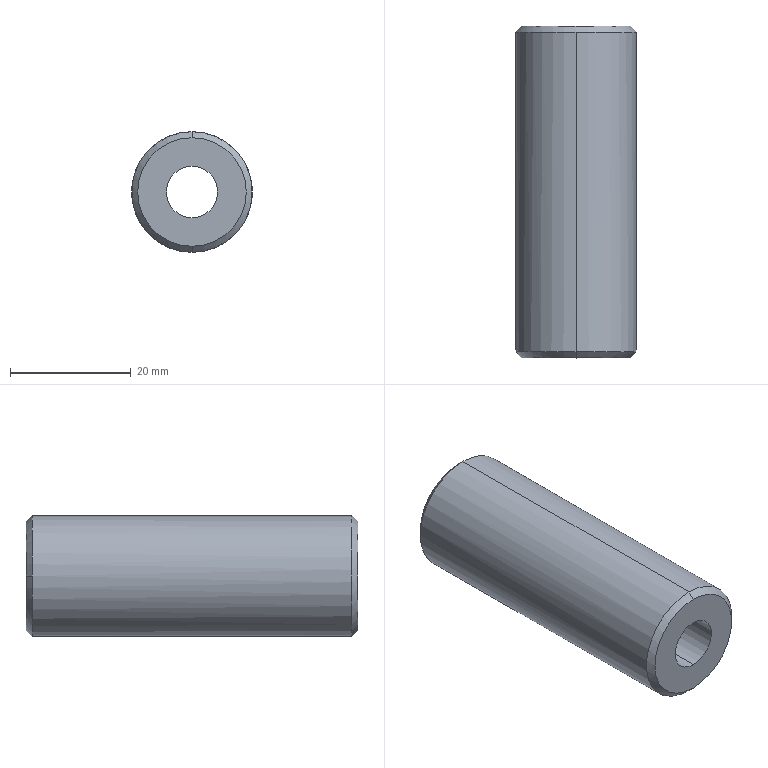Part | SolidWorks | features BaseBody 1 | 1 solid | 10 faces | box 20 x 55 x 20 mm | volume 14097 mm3 | cylinder 4 | cone 4 | plane 2 | commonest cylinder face diameters 8.5 x2 20 x2
STEP:
#1=CARTESIAN_POINT('',(10.,54.,0.));
#2=VERTEX_POINT('',#1);
#3=CARTESIAN_POINT('',(0.,54.,10.));
#4=VERTEX_POINT('',#3);
#5=CARTESIAN_POINT('',(0.,54.,0.));
#6=DIRECTION('',(0.,-1.,0.));
#7=DIRECTION('',(0.,0.,-1.));
#8=AXIS2_PLACEMENT_3D('',#5,#6,#7);
#9=CIRCLE('',#8,10.);
#10=EDGE_CURVE('',#2,#4,#9,.T.);
#11=ORIENTED_EDGE('',*,*,#10,.T.);
#12=CARTESIAN_POINT('',(0.,1.,10.));
#13=VERTEX_POINT('',#12);
#14=CARTESIAN_POINT('',(0.,55.,10.));
#15=DIRECTION('',(0.,-1.,0.));
#16=VECTOR('',#15,1000.);
#17=LINE('',#14,#16);
#18=EDGE_CURVE('',#4,#13,#17,.T.);
#19=ORIENTED_EDGE('',*,*,#18,.T.);
#20=CARTESIAN_POINT('',(0.,1.,-10.));
#21=VERTEX_POINT('',#20);
#22=CARTESIAN_POINT('',(0.,1.,0.));
#23=DIRECTION('',(0.,1.,0.));
#24=DIRECTION('',(0.,0.,-1.));
#25=AXIS2_PLACEMENT_3D('',#22,#23,#24);
#26=CIRCLE('',#25,10.);
#27=EDGE_CURVE('',#13,#21,#26,.T.);
#28=ORIENTED_EDGE('',*,*,#27,.T.);
#29=CARTESIAN_POINT('',(0.,54.,-10.));
#30=VERTEX_POINT('',#29);
#31=CARTESIAN_POINT('',(0.,55.,-10.));
#32=DIRECTION('',(0.,-1.,0.));
#33=VECTOR('',#32,1000.);
#34=LINE('',#31,#33);
#35=EDGE_CURVE('',#30,#21,#34,.T.);
#36=ORIENTED_EDGE('',*,*,#35,.F.);
#37=CARTESIAN_POINT('',(0.,54.,0.));
#38=DIRECTION('',(0.,-1.,0.));
#39=DIRECTION('',(0.,0.,-1.));
#40=AXIS2_PLACEMENT_3D('',#37,#38,#39);
#41=CIRCLE('',#40,10.);
#42=EDGE_CURVE('',#30,#2,#41,.T.);
#43=ORIENTED_EDGE('',*,*,#42,.T.);
#44=EDGE_LOOP('',(#11,#19,#28,#36,#43));
#45=FACE_OUTER_BOUND('',#44,.T.);
#46=CARTESIAN_POINT('',(0.,55.,0.));
#47=DIRECTION('',(0.,-1.,0.));
#48=DIRECTION('',(0.,0.,-1.));
#49=AXIS2_PLACEMENT_3D('',#46,#47,#48);
#50=CYLINDRICAL_SURFACE('',#49,10.);
#51=ADVANCED_FACE('',(#45),#50,.T.);
#52=CARTESIAN_POINT('',(0.,0.,9.));
#53=VERTEX_POINT('',#52);
#54=CARTESIAN_POINT('',(0.,0.,-9.));
#55=VERTEX_POINT('',#54);
#56=CARTESIAN_POINT('',(0.,0.,0.));
#57=DIRECTION('',(0.,1.,0.));
#58=DIRECTION('',(0.,0.,1.));
#59=AXIS2_PLACEMENT_3D('',#56,#57,#58);
#60=CIRCLE('',#59,9.);
#61=EDGE_CURVE('',#53,#55,#60,.T.);
#62=ORIENTED_EDGE('',*,*,#61,.T.);
#63=CARTESIAN_POINT('',(0.,1.,-10.));
#64=DIRECTION('',(0.,0.7071,-0.7071));
#65=VECTOR('',#64,1000.);
#66=LINE('',#63,#65);
#67=EDGE_CURVE('',#55,#21,#66,.T.);
#68=ORIENTED_EDGE('',*,*,#67,.T.);
#69=ORIENTED_EDGE('',*,*,#27,.F.);
#70=CARTESIAN_POINT('',(0.,1.,10.));
#71=DIRECTION('',(0.,0.7071,0.7071));
#72=VECTOR('',#71,1000.);
#73=LINE('',#70,#72);
#74=EDGE_CURVE('',#53,#13,#73,.T.);
#75=ORIENTED_EDGE('',*,*,#74,.F.);
#76=EDGE_LOOP('',(#62,#68,#69,#75));
#77=FACE_OUTER_BOUND('',#76,.T.);
#78=CARTESIAN_POINT('',(0.,1.,0.));
#79=DIRECTION('',(0.,1.,0.));
#80=DIRECTION('',(0.,0.,1.));
#81=AXIS2_PLACEMENT_3D('',#78,#79,#80);
#82=CONICAL_SURFACE('',#81,10.,0.7854);
#83=ADVANCED_FACE('',(#77),#82,.T.);
#84=CARTESIAN_POINT('',(9.,55.,0.));
#85=VERTEX_POINT('',#84);
#86=CARTESIAN_POINT('',(-9.,55.,0.));
#87=VERTEX_POINT('',#86);
#88=CARTESIAN_POINT('',(0.,55.,0.));
#89=DIRECTION('',(0.,-1.,0.));
#90=DIRECTION('',(1.,0.,0.));
#91=AXIS2_PLACEMENT_3D('',#88,#89,#90);
#92=CIRCLE('',#91,9.);
#93=EDGE_CURVE('',#85,#87,#92,.T.);
#94=ORIENTED_EDGE('',*,*,#93,.T.);
#95=CARTESIAN_POINT('',(-10.,54.,0.));
#96=VERTEX_POINT('',#95);
#97=CARTESIAN_POINT('',(-10.,54.,0.));
#98=DIRECTION('',(-0.7071,-0.7071,0.));
#99=VECTOR('',#98,1000.);
#100=LINE('',#97,#99);
#101=EDGE_CURVE('',#87,#96,#100,.T.);
#102=ORIENTED_EDGE('',*,*,#101,.T.);
#103=CARTESIAN_POINT('',(0.,54.,0.));
#104=DIRECTION('',(0.,-1.,0.));
#105=DIRECTION('',(0.,0.,-1.));
#106=AXIS2_PLACEMENT_3D('',#103,#104,#105);
#107=CIRCLE('',#106,10.);
#108=EDGE_CURVE('',#4,#96,#107,.T.);
#109=ORIENTED_EDGE('',*,*,#108,.F.);
#110=ORIENTED_EDGE('',*,*,#10,.F.);
#111=CARTESIAN_POINT('',(10.,54.,0.));
#112=DIRECTION('',(0.7071,-0.7071,0.));
#113=VECTOR('',#112,1000.);
#114=LINE('',#111,#113);
#115=EDGE_CURVE('',#85,#2,#114,.T.);
#116=ORIENTED_EDGE('',*,*,#115,.F.);
#117=EDGE_LOOP('',(#94,#102,#109,#110,#116));
#118=FACE_OUTER_BOUND('',#117,.T.);
#119=CARTESIAN_POINT('',(0.,54.,0.));
#120=DIRECTION('',(0.,-1.,0.));
#121=DIRECTION('',(1.,0.,0.));
#122=AXIS2_PLACEMENT_3D('',#119,#120,#121);
#123=CONICAL_SURFACE('',#122,10.,0.7854);
#124=ADVANCED_FACE('',(#118),#123,.T.);
#125=CARTESIAN_POINT('',(0.,0.,4.25));
#126=VERTEX_POINT('',#125);
#127=CARTESIAN_POINT('',(0.,0.,-4.25));
#128=VERTEX_POINT('',#127);
#129=CARTESIAN_POINT('',(0.,0.,0.));
#130=DIRECTION('',(0.,-1.,0.));
#131=DIRECTION('',(0.,0.,1.));
#132=AXIS2_PLACEMENT_3D('',#129,#130,#131);
#133=CIRCLE('',#132,4.25);
#134=EDGE_CURVE('',#126,#128,#133,.T.);
#135=ORIENTED_EDGE('',*,*,#134,.T.);
#136=CARTESIAN_POINT('',(0.,55.,-4.25));
#137=VERTEX_POINT('',#136);
#138=CARTESIAN_POINT('',(0.,55.,-4.25));
#139=DIRECTION('',(0.,1.,0.));
#140=VECTOR('',#139,1000.);
#141=LINE('',#138,#140);
#142=EDGE_CURVE('',#128,#137,#141,.T.);
#143=ORIENTED_EDGE('',*,*,#142,.T.);
#144=CARTESIAN_POINT('',(0.,55.,4.25));
#145=VERTEX_POINT('',#144);
#146=CARTESIAN_POINT('',(0.,55.,0.));
#147=DIRECTION('',(0.,-1.,0.));
#148=DIRECTION('',(0.,0.,1.));
#149=AXIS2_PLACEMENT_3D('',#146,#147,#148);
#150=CIRCLE('',#149,4.25);
#151=EDGE_CURVE('',#145,#137,#150,.T.);
#152=ORIENTED_EDGE('',*,*,#151,.F.);
#153=CARTESIAN_POINT('',(0.,55.,4.25));
#154=DIRECTION('',(0.,1.,0.));
#155=VECTOR('',#154,1000.);
#156=LINE('',#153,#155);
#157=EDGE_CURVE('',#126,#145,#156,.T.);
#158=ORIENTED_EDGE('',*,*,#157,.F.);
#159=EDGE_LOOP('',(#135,#143,#152,#158));
#160=FACE_OUTER_BOUND('',#159,.T.);
#161=CARTESIAN_POINT('',(0.,55.,0.));
#162=DIRECTION('',(0.,1.,0.));
#163=DIRECTION('',(0.,0.,1.));
#164=AXIS2_PLACEMENT_3D('',#161,#162,#163);
#165=CYLINDRICAL_SURFACE('',#164,4.25);
#166=ADVANCED_FACE('',(#160),#165,.F.);
#167=ORIENTED_EDGE('',*,*,#18,.F.);
#168=ORIENTED_EDGE('',*,*,#108,.T.);
#169=CARTESIAN_POINT('',(0.,54.,0.));
#170=DIRECTION('',(0.,-1.,0.));
#171=DIRECTION('',(0.,0.,-1.));
#172=AXIS2_PLACEMENT_3D('',#169,#170,#171);
#173=CIRCLE('',#172,10.);
#174=EDGE_CURVE('',#96,#30,#173,.T.);
#175=ORIENTED_EDGE('',*,*,#174,.T.);
#176=ORIENTED_EDGE('',*,*,#35,.T.);
#177=CARTESIAN_POINT('',(0.,1.,0.));
#178=DIRECTION('',(0.,1.,0.));
#179=DIRECTION('',(0.,0.,-1.));
#180=AXIS2_PLACEMENT_3D('',#177,#178,#179);
#181=CIRCLE('',#180,10.);
#182=EDGE_CURVE('',#21,#13,#181,.T.);
#183=ORIENTED_EDGE('',*,*,#182,.T.);
#184=EDGE_LOOP('',(#167,#168,#175,#176,#183));
#185=FACE_OUTER_BOUND('',#184,.T.);
#186=CARTESIAN_POINT('',(0.,55.,0.));
#187=DIRECTION('',(0.,-1.,0.));
#188=DIRECTION('',(0.,0.,-1.));
#189=AXIS2_PLACEMENT_3D('',#186,#187,#188);
#190=CYLINDRICAL_SURFACE('',#189,10.);
#191=ADVANCED_FACE('',(#185),#190,.T.);
#192=ORIENTED_EDGE('',*,*,#67,.F.);
#193=CARTESIAN_POINT('',(0.,0.,0.));
#194=DIRECTION('',(0.,1.,0.));
#195=DIRECTION('',(0.,0.,1.));
#196=AXIS2_PLACEMENT_3D('',#193,#194,#195);
#197=CIRCLE('',#196,9.);
#198=EDGE_CURVE('',#55,#53,#197,.T.);
#199=ORIENTED_EDGE('',*,*,#198,.T.);
#200=ORIENTED_EDGE('',*,*,#74,.T.);
#201=ORIENTED_EDGE('',*,*,#182,.F.);
#202=EDGE_LOOP('',(#192,#199,#200,#201));
#203=FACE_OUTER_BOUND('',#202,.T.);
#204=CARTESIAN_POINT('',(0.,1.,0.));
#205=DIRECTION('',(0.,1.,0.));
#206=DIRECTION('',(0.,0.,1.));
#207=AXIS2_PLACEMENT_3D('',#204,#205,#206);
#208=CONICAL_SURFACE('',#207,10.,0.7854);
#209=ADVANCED_FACE('',(#203),#208,.T.);
#210=ORIENTED_EDGE('',*,*,#101,.F.);
#211=CARTESIAN_POINT('',(0.,55.,0.));
#212=DIRECTION('',(0.,-1.,0.));
#213=DIRECTION('',(1.,0.,0.));
#214=AXIS2_PLACEMENT_3D('',#211,#212,#213);
#215=CIRCLE('',#214,9.);
#216=EDGE_CURVE('',#87,#85,#215,.T.);
#217=ORIENTED_EDGE('',*,*,#216,.T.);
#218=ORIENTED_EDGE('',*,*,#115,.T.);
#219=ORIENTED_EDGE('',*,*,#42,.F.);
#220=ORIENTED_EDGE('',*,*,#174,.F.);
#221=EDGE_LOOP('',(#210,#217,#218,#219,#220));
#222=FACE_OUTER_BOUND('',#221,.T.);
#223=CARTESIAN_POINT('',(0.,54.,0.));
#224=DIRECTION('',(0.,-1.,0.));
#225=DIRECTION('',(1.,0.,0.));
#226=AXIS2_PLACEMENT_3D('',#223,#224,#225);
#227=CONICAL_SURFACE('',#226,10.,0.7854);
#228=ADVANCED_FACE('',(#222),#227,.T.);
#229=ORIENTED_EDGE('',*,*,#134,.F.);
#230=CARTESIAN_POINT('',(0.,0.,0.));
#231=DIRECTION('',(0.,-1.,0.));
#232=DIRECTION('',(0.,0.,1.));
#233=AXIS2_PLACEMENT_3D('',#230,#231,#232);
#234=CIRCLE('',#233,4.25);
#235=EDGE_CURVE('',#128,#126,#234,.T.);
#236=ORIENTED_EDGE('',*,*,#235,.F.);
#237=EDGE_LOOP('',(#229,#236));
#238=FACE_BOUND('',#237,.T.);
#239=ORIENTED_EDGE('',*,*,#61,.F.);
#240=ORIENTED_EDGE('',*,*,#198,.F.);
#241=EDGE_LOOP('',(#239,#240));
#242=FACE_OUTER_BOUND('',#241,.T.);
#243=CARTESIAN_POINT('',(0.,0.,0.));
#244=DIRECTION('',(0.,1.,0.));
#245=DIRECTION('',(0.,0.,1.));
#246=AXIS2_PLACEMENT_3D('',#243,#244,#245);
#247=PLANE('',#246);
#248=ADVANCED_FACE('',(#238,#242),#247,.F.);
#249=ORIENTED_EDGE('',*,*,#151,.T.);
#250=CARTESIAN_POINT('',(0.,55.,0.));
#251=DIRECTION('',(0.,-1.,0.));
#252=DIRECTION('',(0.,0.,1.));
#253=AXIS2_PLACEMENT_3D('',#250,#251,#252);
#254=CIRCLE('',#253,4.25);
#255=EDGE_CURVE('',#137,#145,#254,.T.);
#256=ORIENTED_EDGE('',*,*,#255,.T.);
#257=EDGE_LOOP('',(#249,#256));
#258=FACE_BOUND('',#257,.T.);
#259=ORIENTED_EDGE('',*,*,#93,.F.);
#260=ORIENTED_EDGE('',*,*,#216,.F.);
#261=EDGE_LOOP('',(#259,#260));
#262=FACE_OUTER_BOUND('',#261,.T.);
#263=CARTESIAN_POINT('',(0.,55.,0.));
#264=DIRECTION('',(0.,1.,0.));
#265=DIRECTION('',(0.,0.,1.));
#266=AXIS2_PLACEMENT_3D('',#263,#264,#265);
#267=PLANE('',#266);
#268=ADVANCED_FACE('',(#258,#262),#267,.T.);
#269=ORIENTED_EDGE('',*,*,#142,.F.);
#270=ORIENTED_EDGE('',*,*,#235,.T.);
#271=ORIENTED_EDGE('',*,*,#157,.T.);
#272=ORIENTED_EDGE('',*,*,#255,.F.);
#273=EDGE_LOOP('',(#269,#270,#271,#272));
#274=FACE_OUTER_BOUND('',#273,.T.);
#275=CARTESIAN_POINT('',(0.,55.,0.));
#276=DIRECTION('',(0.,1.,0.));
#277=DIRECTION('',(0.,0.,1.));
#278=AXIS2_PLACEMENT_3D('',#275,#276,#277);
#279=CYLINDRICAL_SURFACE('',#278,4.25);
#280=ADVANCED_FACE('',(#274),#279,.F.);
#281=CLOSED_SHELL('',(#51,#83,#124,#166,#191,#209,#228,#248,#268,#280));
#282=MANIFOLD_SOLID_BREP('',#281);
#283=CARTESIAN_POINT('',(0.,0.,0.));
#284=DIRECTION('',(0.,0.,1.));
#285=DIRECTION('',(1.,0.,0.));
#286=AXIS2_PLACEMENT_3D('',#283,#284,#285);
#287=(LENGTH_UNIT()NAMED_UNIT(*)SI_UNIT(.MILLI.,.METRE.));
#288=UNCERTAINTY_MEASURE_WITH_UNIT(LENGTH_MEASURE(0.00001),#287,'','');
#289=(NAMED_UNIT(*)PLANE_ANGLE_UNIT()SI_UNIT($,.RADIAN.));
#290=(NAMED_UNIT(*)SI_UNIT($,.STERADIAN.)SOLID_ANGLE_UNIT());
#291=(GEOMETRIC_REPRESENTATION_CONTEXT(3)GLOBAL_UNCERTAINTY_ASSIGNED_CONTEXT((#288))GLOBAL_UNIT_ASSIGNED_CONTEXT((#287,#289,#290))REPRESENTATION_CONTEXT('',''));
#292=ADVANCED_BREP_SHAPE_REPRESENTATION('',(#282,#286),#291);